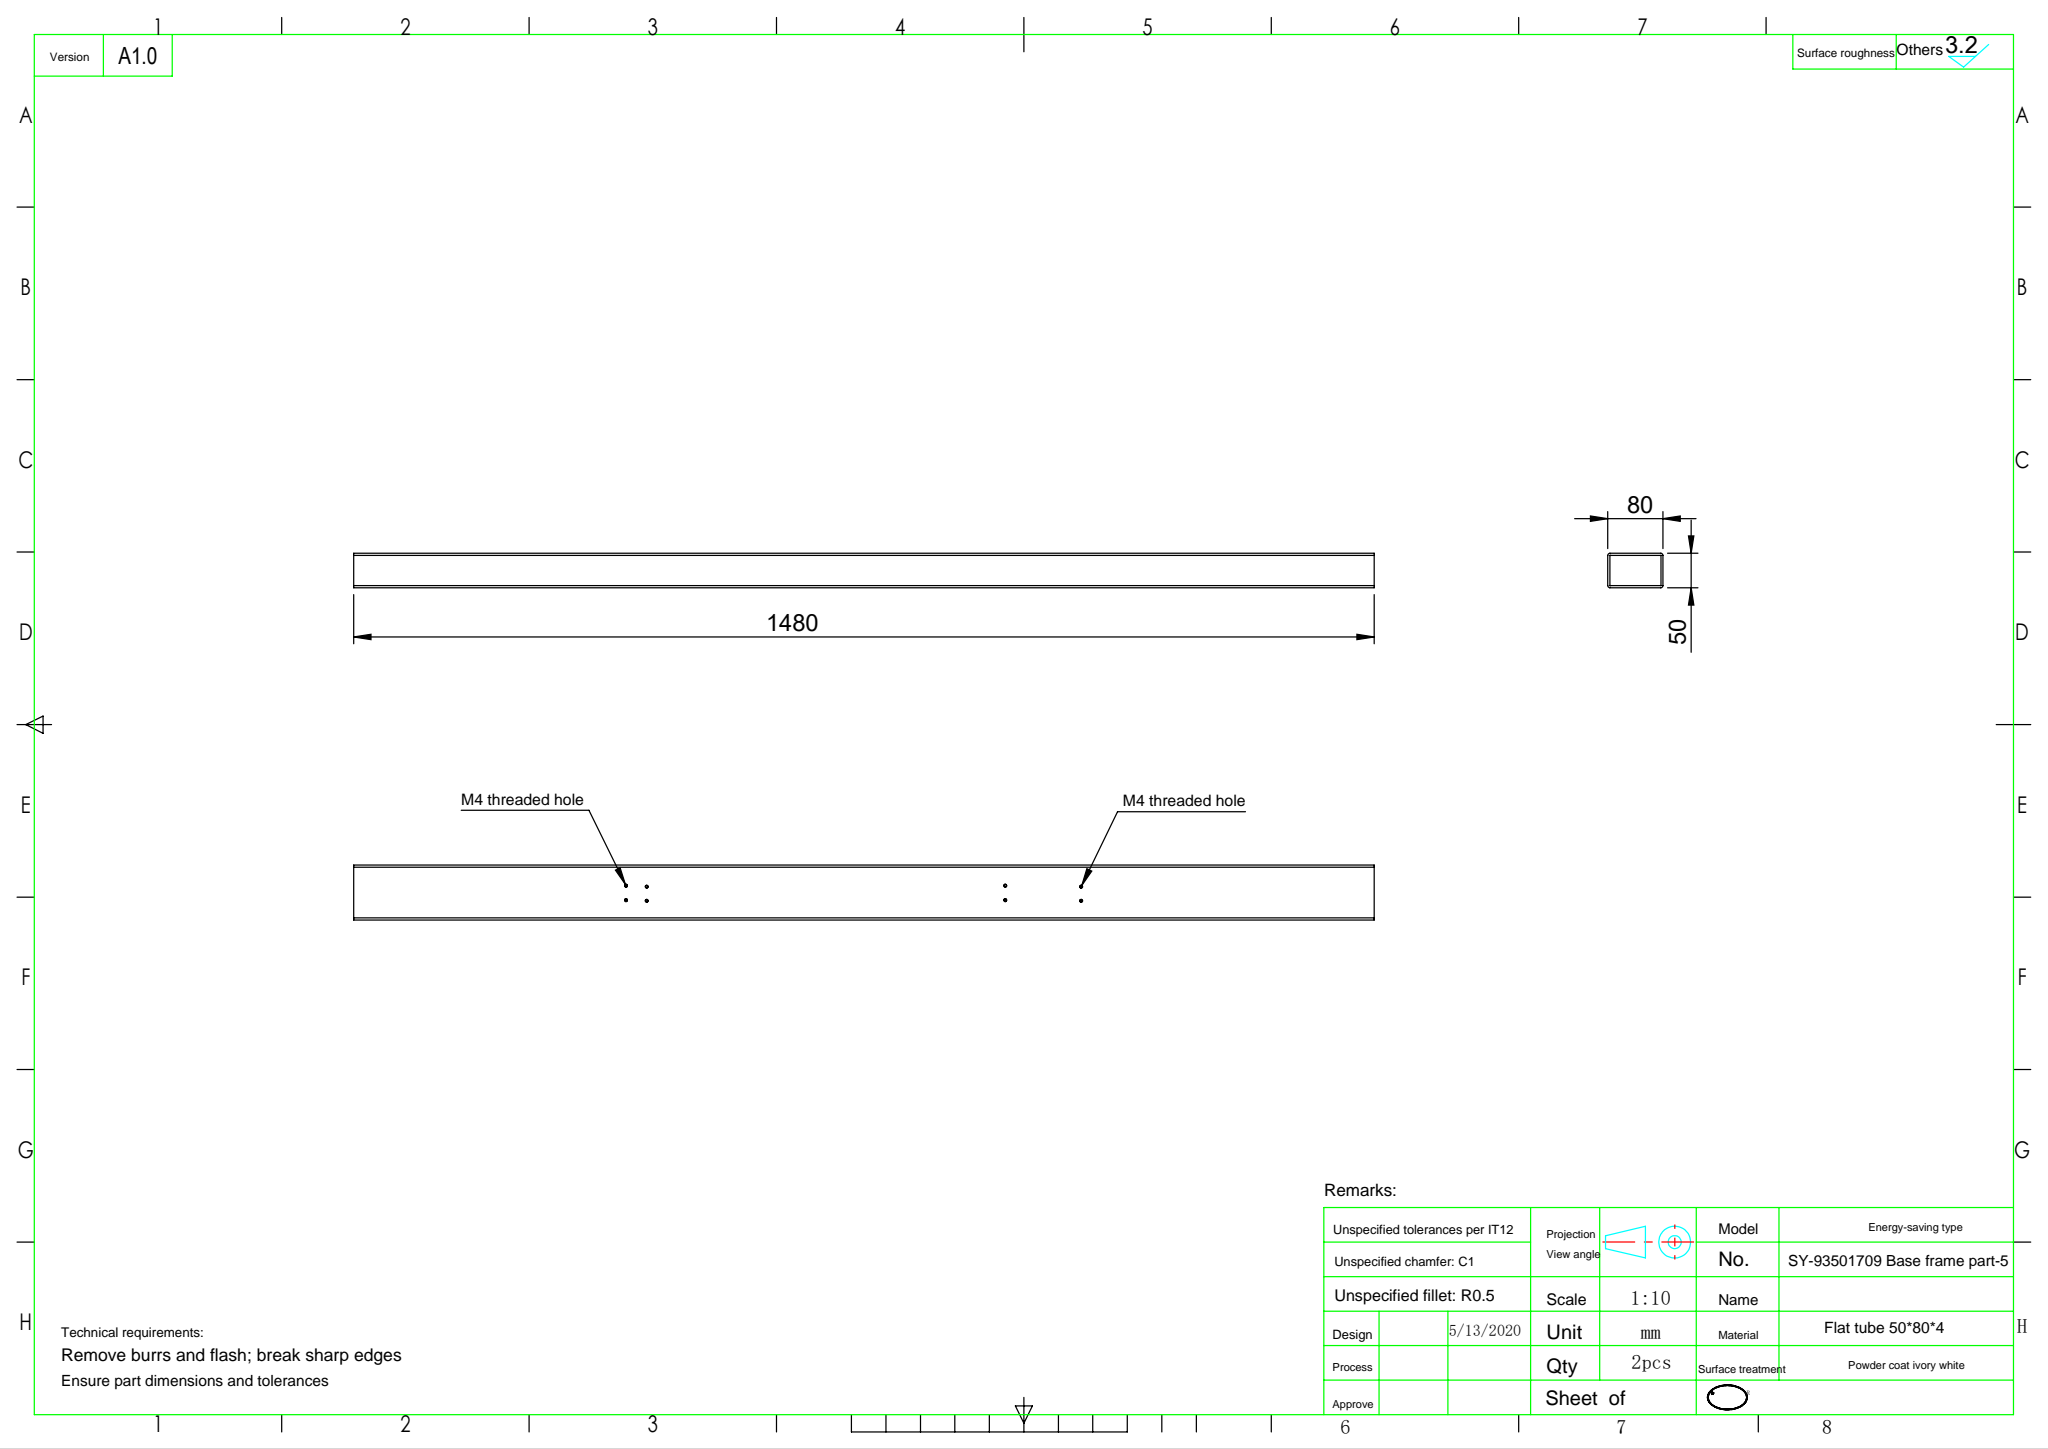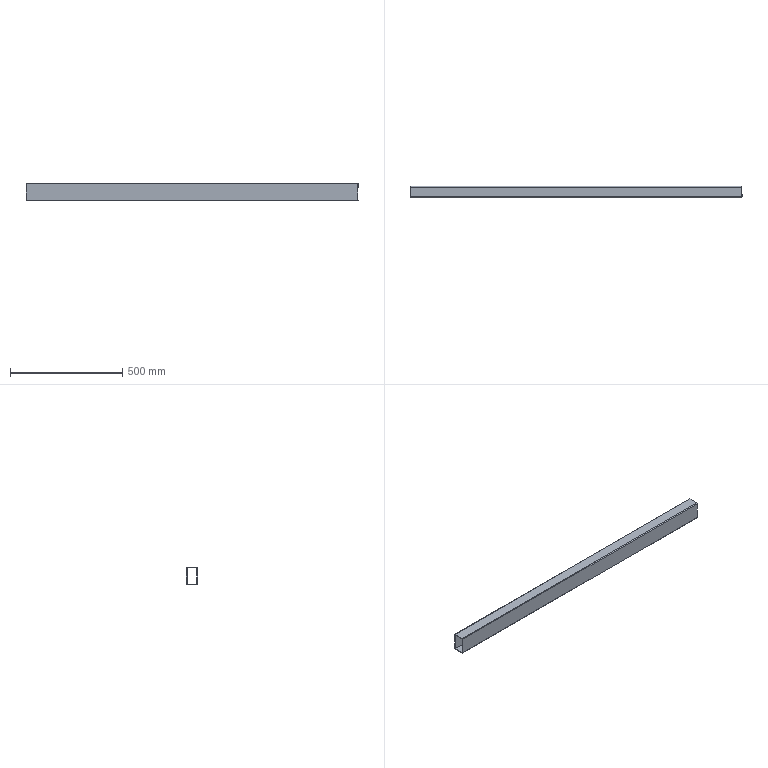Part | SolidWorks | features HoleWzd 2, BaseBody 1, ICE 1, MoveFace 1 | 1 solid | 50 faces | box 1480 x 50 x 80 mm | volume 1087950 mm3 | cylinder 24 | cone 16 | plane 10 | commonest cylinder face diameters 3.3 x16 0.4 x4 6.4 x4